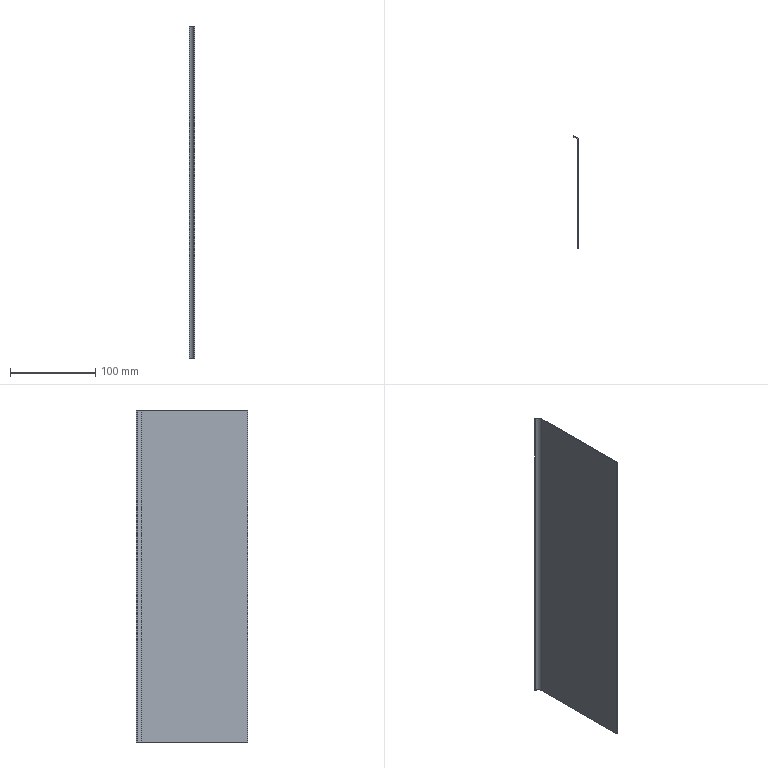Part | SolidWorks | features BaseBody 1 | 1 solid | 10 faces | box 6 x 131 x 390 mm | volume 52119 mm3 | plane 8 | cylinder 2 | commonest cylinder face diameters 10 x1 12 x1
STEP:
#1=CARTESIAN_POINT('',(1.,125.,195.));
#2=VERTEX_POINT('',#1);
#3=CARTESIAN_POINT('',(0.,125.,195.));
#4=VERTEX_POINT('',#3);
#5=CARTESIAN_POINT('',(1.,125.,195.));
#6=DIRECTION('',(-1.,0.,0.));
#7=VECTOR('',#6,1000.);
#8=LINE('',#5,#7);
#9=EDGE_CURVE('',#2,#4,#8,.T.);
#10=ORIENTED_EDGE('',*,*,#9,.F.);
#11=CARTESIAN_POINT('',(-5.,131.,195.));
#12=VERTEX_POINT('',#11);
#13=CARTESIAN_POINT('',(-5.,125.,195.));
#14=DIRECTION('',(0.,0.,1.));
#15=DIRECTION('',(1.,0.,0.));
#16=AXIS2_PLACEMENT_3D('',#13,#14,#15);
#17=CIRCLE('',#16,6.);
#18=EDGE_CURVE('',#2,#12,#17,.T.);
#19=ORIENTED_EDGE('',*,*,#18,.T.);
#20=CARTESIAN_POINT('',(-5.,130.,195.));
#21=VERTEX_POINT('',#20);
#22=CARTESIAN_POINT('',(-5.,130.,195.));
#23=DIRECTION('',(0.,1.,0.));
#24=VECTOR('',#23,1000.);
#25=LINE('',#22,#24);
#26=EDGE_CURVE('',#21,#12,#25,.T.);
#27=ORIENTED_EDGE('',*,*,#26,.F.);
#28=CARTESIAN_POINT('',(-5.,125.,195.));
#29=DIRECTION('',(0.,0.,1.));
#30=DIRECTION('',(1.,0.,0.));
#31=AXIS2_PLACEMENT_3D('',#28,#29,#30);
#32=CIRCLE('',#31,5.);
#33=EDGE_CURVE('',#4,#21,#32,.T.);
#34=ORIENTED_EDGE('',*,*,#33,.F.);
#35=EDGE_LOOP('',(#10,#19,#27,#34));
#36=FACE_OUTER_BOUND('',#35,.T.);
#37=CARTESIAN_POINT('',(1.,125.,195.));
#38=DIRECTION('',(0.,0.,1.));
#39=DIRECTION('',(1.,0.,0.));
#40=AXIS2_PLACEMENT_3D('',#37,#38,#39);
#41=PLANE('',#40);
#42=ADVANCED_FACE('',(#36),#41,.T.);
#43=CARTESIAN_POINT('',(0.,125.,-195.));
#44=VERTEX_POINT('',#43);
#45=CARTESIAN_POINT('',(1.,125.,-195.));
#46=VERTEX_POINT('',#45);
#47=CARTESIAN_POINT('',(0.,125.,-195.));
#48=DIRECTION('',(1.,0.,0.));
#49=VECTOR('',#48,1000.);
#50=LINE('',#47,#49);
#51=EDGE_CURVE('',#44,#46,#50,.T.);
#52=ORIENTED_EDGE('',*,*,#51,.F.);
#53=CARTESIAN_POINT('',(-5.,130.,-195.));
#54=VERTEX_POINT('',#53);
#55=CARTESIAN_POINT('',(-5.,125.,-195.));
#56=DIRECTION('',(0.,0.,1.));
#57=DIRECTION('',(1.,0.,0.));
#58=AXIS2_PLACEMENT_3D('',#55,#56,#57);
#59=CIRCLE('',#58,5.);
#60=EDGE_CURVE('',#44,#54,#59,.T.);
#61=ORIENTED_EDGE('',*,*,#60,.T.);
#62=CARTESIAN_POINT('',(-5.,131.,-195.));
#63=VERTEX_POINT('',#62);
#64=CARTESIAN_POINT('',(-5.,130.,-195.));
#65=DIRECTION('',(0.,1.,0.));
#66=VECTOR('',#65,1000.);
#67=LINE('',#64,#66);
#68=EDGE_CURVE('',#54,#63,#67,.T.);
#69=ORIENTED_EDGE('',*,*,#68,.T.);
#70=CARTESIAN_POINT('',(-5.,125.,-195.));
#71=DIRECTION('',(0.,0.,1.));
#72=DIRECTION('',(1.,0.,0.));
#73=AXIS2_PLACEMENT_3D('',#70,#71,#72);
#74=CIRCLE('',#73,6.);
#75=EDGE_CURVE('',#46,#63,#74,.T.);
#76=ORIENTED_EDGE('',*,*,#75,.F.);
#77=EDGE_LOOP('',(#52,#61,#69,#76));
#78=FACE_OUTER_BOUND('',#77,.T.);
#79=CARTESIAN_POINT('',(0.,125.,-195.));
#80=DIRECTION('',(0.,0.,-1.));
#81=DIRECTION('',(-1.,0.,0.));
#82=AXIS2_PLACEMENT_3D('',#79,#80,#81);
#83=PLANE('',#82);
#84=ADVANCED_FACE('',(#78),#83,.T.);
#85=ORIENTED_EDGE('',*,*,#75,.T.);
#86=CARTESIAN_POINT('',(-5.,131.,195.));
#87=DIRECTION('',(0.,0.,-1.));
#88=VECTOR('',#87,1000.);
#89=LINE('',#86,#88);
#90=EDGE_CURVE('',#12,#63,#89,.T.);
#91=ORIENTED_EDGE('',*,*,#90,.F.);
#92=ORIENTED_EDGE('',*,*,#18,.F.);
#93=CARTESIAN_POINT('',(1.,125.,195.));
#94=DIRECTION('',(0.,0.,-1.));
#95=VECTOR('',#94,1000.);
#96=LINE('',#93,#95);
#97=EDGE_CURVE('',#2,#46,#96,.T.);
#98=ORIENTED_EDGE('',*,*,#97,.T.);
#99=EDGE_LOOP('',(#85,#91,#92,#98));
#100=FACE_OUTER_BOUND('',#99,.T.);
#101=CARTESIAN_POINT('',(-5.,125.,195.));
#102=DIRECTION('',(0.,0.,-1.));
#103=DIRECTION('',(-1.,0.,0.));
#104=AXIS2_PLACEMENT_3D('',#101,#102,#103);
#105=CYLINDRICAL_SURFACE('',#104,6.);
#106=ADVANCED_FACE('',(#100),#105,.T.);
#107=ORIENTED_EDGE('',*,*,#68,.F.);
#108=CARTESIAN_POINT('',(-5.,130.,195.));
#109=DIRECTION('',(0.,0.,-1.));
#110=VECTOR('',#109,1000.);
#111=LINE('',#108,#110);
#112=EDGE_CURVE('',#21,#54,#111,.T.);
#113=ORIENTED_EDGE('',*,*,#112,.F.);
#114=ORIENTED_EDGE('',*,*,#26,.T.);
#115=ORIENTED_EDGE('',*,*,#90,.T.);
#116=EDGE_LOOP('',(#107,#113,#114,#115));
#117=FACE_OUTER_BOUND('',#116,.T.);
#118=CARTESIAN_POINT('',(-5.,130.,195.));
#119=DIRECTION('',(-1.,0.,0.));
#120=DIRECTION('',(0.,0.,1.));
#121=AXIS2_PLACEMENT_3D('',#118,#119,#120);
#122=PLANE('',#121);
#123=ADVANCED_FACE('',(#117),#122,.T.);
#124=ORIENTED_EDGE('',*,*,#60,.F.);
#125=CARTESIAN_POINT('',(0.,125.,195.));
#126=DIRECTION('',(0.,0.,-1.));
#127=VECTOR('',#126,1000.);
#128=LINE('',#125,#127);
#129=EDGE_CURVE('',#4,#44,#128,.T.);
#130=ORIENTED_EDGE('',*,*,#129,.F.);
#131=ORIENTED_EDGE('',*,*,#33,.T.);
#132=ORIENTED_EDGE('',*,*,#112,.T.);
#133=EDGE_LOOP('',(#124,#130,#131,#132));
#134=FACE_OUTER_BOUND('',#133,.T.);
#135=CARTESIAN_POINT('',(-5.,125.,195.));
#136=DIRECTION('',(0.,0.,-1.));
#137=DIRECTION('',(-1.,0.,0.));
#138=AXIS2_PLACEMENT_3D('',#135,#136,#137);
#139=CYLINDRICAL_SURFACE('',#138,5.);
#140=ADVANCED_FACE('',(#134),#139,.F.);
#141=CARTESIAN_POINT('',(0.,0.,-195.));
#142=VERTEX_POINT('',#141);
#143=CARTESIAN_POINT('',(0.,125.,-195.));
#144=DIRECTION('',(0.,1.,0.));
#145=VECTOR('',#144,1000.);
#146=LINE('',#143,#145);
#147=EDGE_CURVE('',#142,#44,#146,.T.);
#148=ORIENTED_EDGE('',*,*,#147,.F.);
#149=CARTESIAN_POINT('',(0.,0.,195.));
#150=VERTEX_POINT('',#149);
#151=CARTESIAN_POINT('',(0.,0.,195.));
#152=DIRECTION('',(0.,0.,-1.));
#153=VECTOR('',#152,1000.);
#154=LINE('',#151,#153);
#155=EDGE_CURVE('',#150,#142,#154,.T.);
#156=ORIENTED_EDGE('',*,*,#155,.F.);
#157=CARTESIAN_POINT('',(0.,125.,195.));
#158=DIRECTION('',(0.,1.,0.));
#159=VECTOR('',#158,1000.);
#160=LINE('',#157,#159);
#161=EDGE_CURVE('',#150,#4,#160,.T.);
#162=ORIENTED_EDGE('',*,*,#161,.T.);
#163=ORIENTED_EDGE('',*,*,#129,.T.);
#164=EDGE_LOOP('',(#148,#156,#162,#163));
#165=FACE_OUTER_BOUND('',#164,.T.);
#166=CARTESIAN_POINT('',(0.,125.,195.));
#167=DIRECTION('',(-1.,0.,0.));
#168=DIRECTION('',(0.,-1.,0.));
#169=AXIS2_PLACEMENT_3D('',#166,#167,#168);
#170=PLANE('',#169);
#171=ADVANCED_FACE('',(#165),#170,.T.);
#172=CARTESIAN_POINT('',(1.,0.,-195.));
#173=VERTEX_POINT('',#172);
#174=CARTESIAN_POINT('',(1.,0.,-195.));
#175=DIRECTION('',(-1.,0.,0.));
#176=VECTOR('',#175,1000.);
#177=LINE('',#174,#176);
#178=EDGE_CURVE('',#173,#142,#177,.T.);
#179=ORIENTED_EDGE('',*,*,#178,.F.);
#180=CARTESIAN_POINT('',(1.,0.,195.));
#181=VERTEX_POINT('',#180);
#182=CARTESIAN_POINT('',(1.,0.,195.));
#183=DIRECTION('',(0.,0.,-1.));
#184=VECTOR('',#183,1000.);
#185=LINE('',#182,#184);
#186=EDGE_CURVE('',#181,#173,#185,.T.);
#187=ORIENTED_EDGE('',*,*,#186,.F.);
#188=CARTESIAN_POINT('',(1.,0.,195.));
#189=DIRECTION('',(-1.,0.,0.));
#190=VECTOR('',#189,1000.);
#191=LINE('',#188,#190);
#192=EDGE_CURVE('',#181,#150,#191,.T.);
#193=ORIENTED_EDGE('',*,*,#192,.T.);
#194=ORIENTED_EDGE('',*,*,#155,.T.);
#195=EDGE_LOOP('',(#179,#187,#193,#194));
#196=FACE_OUTER_BOUND('',#195,.T.);
#197=CARTESIAN_POINT('',(1.,0.,195.));
#198=DIRECTION('',(0.,-1.,0.));
#199=DIRECTION('',(0.,0.,-1.));
#200=AXIS2_PLACEMENT_3D('',#197,#198,#199);
#201=PLANE('',#200);
#202=ADVANCED_FACE('',(#196),#201,.T.);
#203=CARTESIAN_POINT('',(1.,125.,-195.));
#204=DIRECTION('',(0.,1.,0.));
#205=VECTOR('',#204,1000.);
#206=LINE('',#203,#205);
#207=EDGE_CURVE('',#173,#46,#206,.T.);
#208=ORIENTED_EDGE('',*,*,#207,.T.);
#209=ORIENTED_EDGE('',*,*,#97,.F.);
#210=CARTESIAN_POINT('',(1.,125.,195.));
#211=DIRECTION('',(0.,1.,0.));
#212=VECTOR('',#211,1000.);
#213=LINE('',#210,#212);
#214=EDGE_CURVE('',#181,#2,#213,.T.);
#215=ORIENTED_EDGE('',*,*,#214,.F.);
#216=ORIENTED_EDGE('',*,*,#186,.T.);
#217=EDGE_LOOP('',(#208,#209,#215,#216));
#218=FACE_OUTER_BOUND('',#217,.T.);
#219=CARTESIAN_POINT('',(1.,125.,195.));
#220=DIRECTION('',(-1.,0.,0.));
#221=DIRECTION('',(0.,-1.,0.));
#222=AXIS2_PLACEMENT_3D('',#219,#220,#221);
#223=PLANE('',#222);
#224=ADVANCED_FACE('',(#218),#223,.F.);
#225=ORIENTED_EDGE('',*,*,#214,.T.);
#226=ORIENTED_EDGE('',*,*,#9,.T.);
#227=ORIENTED_EDGE('',*,*,#161,.F.);
#228=ORIENTED_EDGE('',*,*,#192,.F.);
#229=EDGE_LOOP('',(#225,#226,#227,#228));
#230=FACE_OUTER_BOUND('',#229,.T.);
#231=CARTESIAN_POINT('',(-5.,125.,195.));
#232=DIRECTION('',(0.,0.,1.));
#233=DIRECTION('',(1.,0.,0.));
#234=AXIS2_PLACEMENT_3D('',#231,#232,#233);
#235=PLANE('',#234);
#236=ADVANCED_FACE('',(#230),#235,.T.);
#237=ORIENTED_EDGE('',*,*,#147,.T.);
#238=ORIENTED_EDGE('',*,*,#51,.T.);
#239=ORIENTED_EDGE('',*,*,#207,.F.);
#240=ORIENTED_EDGE('',*,*,#178,.T.);
#241=EDGE_LOOP('',(#237,#238,#239,#240));
#242=FACE_OUTER_BOUND('',#241,.T.);
#243=CARTESIAN_POINT('',(-5.,125.,-195.));
#244=DIRECTION('',(0.,0.,1.));
#245=DIRECTION('',(1.,0.,0.));
#246=AXIS2_PLACEMENT_3D('',#243,#244,#245);
#247=PLANE('',#246);
#248=ADVANCED_FACE('',(#242),#247,.F.);
#249=CLOSED_SHELL('',(#42,#84,#106,#123,#140,#171,#202,#224,#236,#248));
#250=MANIFOLD_SOLID_BREP('',#249);
#251=CARTESIAN_POINT('',(0.,0.,0.));
#252=DIRECTION('',(0.,0.,1.));
#253=DIRECTION('',(1.,0.,0.));
#254=AXIS2_PLACEMENT_3D('',#251,#252,#253);
#255=(LENGTH_UNIT()NAMED_UNIT(*)SI_UNIT(.MILLI.,.METRE.));
#256=UNCERTAINTY_MEASURE_WITH_UNIT(LENGTH_MEASURE(0.00001),#255,'','');
#257=(NAMED_UNIT(*)PLANE_ANGLE_UNIT()SI_UNIT($,.RADIAN.));
#258=(NAMED_UNIT(*)SI_UNIT($,.STERADIAN.)SOLID_ANGLE_UNIT());
#259=(GEOMETRIC_REPRESENTATION_CONTEXT(3)GLOBAL_UNCERTAINTY_ASSIGNED_CONTEXT((#256))GLOBAL_UNIT_ASSIGNED_CONTEXT((#255,#257,#258))REPRESENTATION_CONTEXT('',''));
#260=ADVANCED_BREP_SHAPE_REPRESENTATION('',(#250,#254),#259);